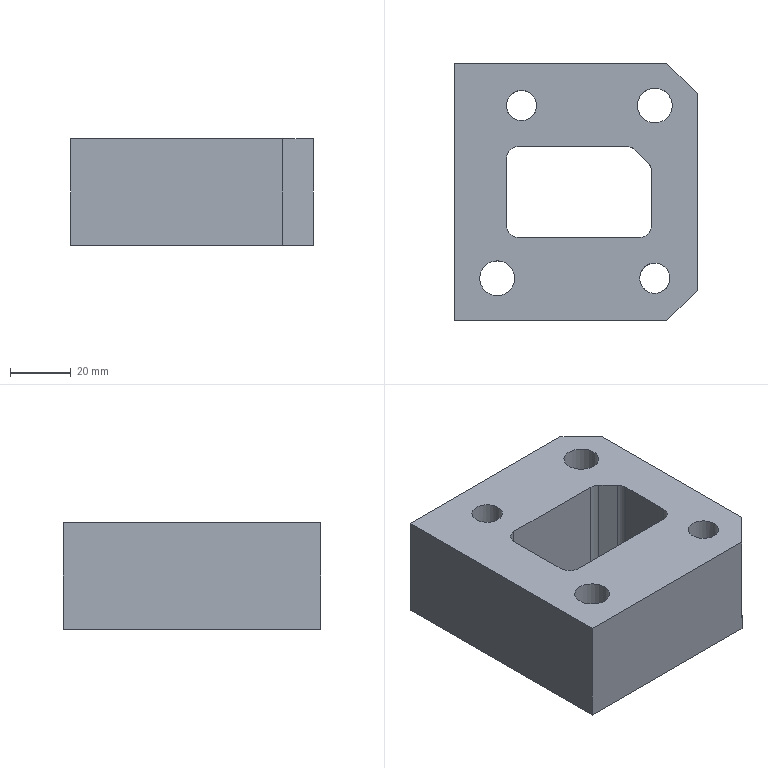Part | NX | features 7 2 | 1 solid | 30 faces | box 80 x 85 x 35 mm | volume 168471 mm3 | plane 17 | cylinder 13 | commonest cylinder face diameters 8 x5 10.001 x2 10.31 x2 11.5 x2 18 x2
STEP:
#1=CARTESIAN_POINT('',(-6.694,33.501,91.));
#2=VERTEX_POINT('',#1);
#3=CARTESIAN_POINT('',(-6.694,28.5,91.));
#4=DIRECTION('',(0.,0.,1.));
#5=DIRECTION('',(0.,1.,0.));
#6=AXIS2_PLACEMENT_3D('',#3,#4,#5);
#7=CIRCLE('',#6,5.);
#8=EDGE_CURVE('',#2,#2,#7,.T.);
#9=ORIENTED_EDGE('',*,*,#8,.F.);
#10=EDGE_LOOP('',(#9));
#11=FACE_BOUND('',#10,.T.);
#12=CARTESIAN_POINT('',(37.306,34.25,91.));
#13=VERTEX_POINT('',#12);
#14=CARTESIAN_POINT('',(37.306,28.5,91.));
#15=DIRECTION('',(0.,0.,-1.));
#16=DIRECTION('',(0.,1.,0.));
#17=AXIS2_PLACEMENT_3D('',#14,#15,#16);
#18=CIRCLE('',#17,5.75);
#19=EDGE_CURVE('',#13,#13,#18,.T.);
#20=ORIENTED_EDGE('',*,*,#19,.T.);
#21=EDGE_LOOP('',(#20));
#22=FACE_BOUND('',#21,.T.);
#23=CARTESIAN_POINT('',(-28.694,-42.5,91.));
#24=VERTEX_POINT('',#23);
#25=CARTESIAN_POINT('',(41.306,-42.5,91.));
#26=VERTEX_POINT('',#25);
#27=CARTESIAN_POINT('',(21.306,-42.5,91.));
#28=DIRECTION('',(1.,0.,0.));
#29=VECTOR('',#28,1000.);
#30=LINE('',#27,#29);
#31=EDGE_CURVE('',#24,#26,#30,.T.);
#32=ORIENTED_EDGE('',*,*,#31,.T.);
#33=CARTESIAN_POINT('',(51.306,-32.5,91.));
#34=VERTEX_POINT('',#33);
#35=CARTESIAN_POINT('',(52.556,-31.25,91.));
#36=DIRECTION('',(0.7071,0.7071,0.));
#37=VECTOR('',#36,1000.);
#38=LINE('',#35,#37);
#39=EDGE_CURVE('',#26,#34,#38,.T.);
#40=ORIENTED_EDGE('',*,*,#39,.T.);
#41=CARTESIAN_POINT('',(51.306,32.5,91.));
#42=VERTEX_POINT('',#41);
#43=CARTESIAN_POINT('',(51.306,0.,91.));
#44=DIRECTION('',(0.,1.,0.));
#45=VECTOR('',#44,1000.);
#46=LINE('',#43,#45);
#47=EDGE_CURVE('',#34,#42,#46,.T.);
#48=ORIENTED_EDGE('',*,*,#47,.T.);
#49=CARTESIAN_POINT('',(41.306,42.5,91.));
#50=VERTEX_POINT('',#49);
#51=CARTESIAN_POINT('',(52.556,31.25,91.));
#52=DIRECTION('',(-0.7071,0.7071,0.));
#53=VECTOR('',#52,1000.);
#54=LINE('',#51,#53);
#55=EDGE_CURVE('',#42,#50,#54,.T.);
#56=ORIENTED_EDGE('',*,*,#55,.T.);
#57=CARTESIAN_POINT('',(-28.694,42.5,91.));
#58=VERTEX_POINT('',#57);
#59=CARTESIAN_POINT('',(21.306,42.5,91.));
#60=DIRECTION('',(-1.,0.,0.));
#61=VECTOR('',#60,1000.);
#62=LINE('',#59,#61);
#63=EDGE_CURVE('',#50,#58,#62,.T.);
#64=ORIENTED_EDGE('',*,*,#63,.T.);
#65=CARTESIAN_POINT('',(-28.694,0.,91.));
#66=DIRECTION('',(0.,-1.,0.));
#67=VECTOR('',#66,1000.);
#68=LINE('',#65,#67);
#69=EDGE_CURVE('',#58,#24,#68,.T.);
#70=ORIENTED_EDGE('',*,*,#69,.T.);
#71=EDGE_LOOP('',(#32,#40,#48,#56,#64,#70));
#72=FACE_BOUND('',#71,.T.);
#73=CARTESIAN_POINT('',(-14.694,-22.75,91.));
#74=VERTEX_POINT('',#73);
#75=CARTESIAN_POINT('',(-14.694,-28.5,91.));
#76=DIRECTION('',(0.,0.,-1.));
#77=DIRECTION('',(0.,1.,0.));
#78=AXIS2_PLACEMENT_3D('',#75,#76,#77);
#79=CIRCLE('',#78,5.75);
#80=EDGE_CURVE('',#74,#74,#79,.T.);
#81=ORIENTED_EDGE('',*,*,#80,.T.);
#82=EDGE_LOOP('',(#81));
#83=FACE_BOUND('',#82,.T.);
#84=CARTESIAN_POINT('',(37.306,-23.499,91.));
#85=VERTEX_POINT('',#84);
#86=CARTESIAN_POINT('',(37.306,-28.5,91.));
#87=DIRECTION('',(0.,0.,1.));
#88=DIRECTION('',(0.,1.,0.));
#89=AXIS2_PLACEMENT_3D('',#86,#87,#88);
#90=CIRCLE('',#89,5.);
#91=EDGE_CURVE('',#85,#85,#90,.T.);
#92=ORIENTED_EDGE('',*,*,#91,.F.);
#93=EDGE_LOOP('',(#92));
#94=FACE_BOUND('',#93,.T.);
#95=CARTESIAN_POINT('',(-7.694,-15.,91.));
#96=VERTEX_POINT('',#95);
#97=CARTESIAN_POINT('',(-11.694,-11.,91.));
#98=VERTEX_POINT('',#97);
#99=CARTESIAN_POINT('',(-7.694,-11.,91.));
#100=DIRECTION('',(0.,0.,-1.));
#101=DIRECTION('',(0.,1.,0.));
#102=AXIS2_PLACEMENT_3D('',#99,#100,#101);
#103=CIRCLE('',#102,4.);
#104=EDGE_CURVE('',#96,#98,#103,.T.);
#105=ORIENTED_EDGE('',*,*,#104,.T.);
#106=CARTESIAN_POINT('',(-11.694,11.,91.));
#107=VERTEX_POINT('',#106);
#108=CARTESIAN_POINT('',(-11.694,0.,91.));
#109=DIRECTION('',(0.,-1.,0.));
#110=VECTOR('',#109,1000.);
#111=LINE('',#108,#110);
#112=EDGE_CURVE('',#107,#98,#111,.T.);
#113=ORIENTED_EDGE('',*,*,#112,.F.);
#114=CARTESIAN_POINT('',(-7.694,15.,91.));
#115=VERTEX_POINT('',#114);
#116=CARTESIAN_POINT('',(-7.694,11.,91.));
#117=DIRECTION('',(0.,0.,-1.));
#118=DIRECTION('',(0.,1.,0.));
#119=AXIS2_PLACEMENT_3D('',#116,#117,#118);
#120=CIRCLE('',#119,4.);
#121=EDGE_CURVE('',#107,#115,#120,.T.);
#122=ORIENTED_EDGE('',*,*,#121,.T.);
#123=CARTESIAN_POINT('',(28.013,15.,91.));
#124=VERTEX_POINT('',#123);
#125=CARTESIAN_POINT('',(21.306,15.,91.));
#126=DIRECTION('',(-1.,0.,0.));
#127=VECTOR('',#126,1000.);
#128=LINE('',#125,#127);
#129=EDGE_CURVE('',#124,#115,#128,.T.);
#130=ORIENTED_EDGE('',*,*,#129,.F.);
#131=CARTESIAN_POINT('',(30.842,13.828,91.));
#132=VERTEX_POINT('',#131);
#133=CARTESIAN_POINT('',(28.013,11.,91.));
#134=DIRECTION('',(0.,0.,-1.));
#135=DIRECTION('',(0.,1.,0.));
#136=AXIS2_PLACEMENT_3D('',#133,#134,#135);
#137=CIRCLE('',#136,4.);
#138=EDGE_CURVE('',#124,#132,#137,.T.);
#139=ORIENTED_EDGE('',*,*,#138,.T.);
#140=CARTESIAN_POINT('',(35.135,9.536,91.));
#141=VERTEX_POINT('',#140);
#142=CARTESIAN_POINT('',(31.738,12.932,91.));
#143=DIRECTION('',(0.7071,-0.7071,0.));
#144=VECTOR('',#143,1000.);
#145=LINE('',#142,#144);
#146=EDGE_CURVE('',#132,#141,#145,.T.);
#147=ORIENTED_EDGE('',*,*,#146,.T.);
#148=CARTESIAN_POINT('',(36.306,6.707,91.));
#149=VERTEX_POINT('',#148);
#150=CARTESIAN_POINT('',(32.306,6.707,91.));
#151=DIRECTION('',(0.,0.,-1.));
#152=DIRECTION('',(0.,1.,0.));
#153=AXIS2_PLACEMENT_3D('',#150,#151,#152);
#154=CIRCLE('',#153,4.);
#155=EDGE_CURVE('',#141,#149,#154,.T.);
#156=ORIENTED_EDGE('',*,*,#155,.T.);
#157=CARTESIAN_POINT('',(36.306,-11.,91.));
#158=VERTEX_POINT('',#157);
#159=CARTESIAN_POINT('',(36.306,0.,91.));
#160=DIRECTION('',(0.,1.,0.));
#161=VECTOR('',#160,1000.);
#162=LINE('',#159,#161);
#163=EDGE_CURVE('',#158,#149,#162,.T.);
#164=ORIENTED_EDGE('',*,*,#163,.F.);
#165=CARTESIAN_POINT('',(32.306,-15.,91.));
#166=VERTEX_POINT('',#165);
#167=CARTESIAN_POINT('',(32.306,-11.,91.));
#168=DIRECTION('',(0.,0.,-1.));
#169=DIRECTION('',(0.,1.,0.));
#170=AXIS2_PLACEMENT_3D('',#167,#168,#169);
#171=CIRCLE('',#170,4.);
#172=EDGE_CURVE('',#158,#166,#171,.T.);
#173=ORIENTED_EDGE('',*,*,#172,.T.);
#174=CARTESIAN_POINT('',(21.306,-15.,91.));
#175=DIRECTION('',(1.,0.,0.));
#176=VECTOR('',#175,1000.);
#177=LINE('',#174,#176);
#178=EDGE_CURVE('',#96,#166,#177,.T.);
#179=ORIENTED_EDGE('',*,*,#178,.F.);
#180=EDGE_LOOP('',(#105,#113,#122,#130,#139,#147,#156,#164,#173,#179));
#181=FACE_BOUND('',#180,.T.);
#182=CARTESIAN_POINT('',(21.306,0.,91.));
#183=DIRECTION('',(0.,0.,1.));
#184=DIRECTION('',(0.,-1.,0.));
#185=AXIS2_PLACEMENT_3D('',#182,#183,#184);
#186=PLANE('',#185);
#187=ADVANCED_FACE('',(#11,#22,#72,#83,#94,#181),#186,.T.);
#188=CARTESIAN_POINT('',(42.461,-28.5,56.));
#189=VERTEX_POINT('',#188);
#190=CARTESIAN_POINT('',(37.306,-28.5,56.));
#191=DIRECTION('',(0.,0.,1.));
#192=DIRECTION('',(1.,0.,0.));
#193=AXIS2_PLACEMENT_3D('',#190,#191,#192);
#194=CIRCLE('',#193,5.155);
#195=EDGE_CURVE('',#189,#189,#194,.T.);
#196=ORIENTED_EDGE('',*,*,#195,.T.);
#197=EDGE_LOOP('',(#196));
#198=FACE_BOUND('',#197,.T.);
#199=CARTESIAN_POINT('',(-1.539,28.5,56.));
#200=VERTEX_POINT('',#199);
#201=CARTESIAN_POINT('',(-6.694,28.5,56.));
#202=DIRECTION('',(0.,0.,1.));
#203=DIRECTION('',(1.,0.,0.));
#204=AXIS2_PLACEMENT_3D('',#201,#202,#203);
#205=CIRCLE('',#204,5.155);
#206=EDGE_CURVE('',#200,#200,#205,.T.);
#207=ORIENTED_EDGE('',*,*,#206,.T.);
#208=EDGE_LOOP('',(#207));
#209=FACE_BOUND('',#208,.T.);
#210=CARTESIAN_POINT('',(51.306,32.5,56.));
#211=VERTEX_POINT('',#210);
#212=CARTESIAN_POINT('',(51.306,-32.5,56.));
#213=VERTEX_POINT('',#212);
#214=CARTESIAN_POINT('',(51.306,0.,56.));
#215=DIRECTION('',(0.,-1.,0.));
#216=VECTOR('',#215,1000.);
#217=LINE('',#214,#216);
#218=EDGE_CURVE('',#211,#213,#217,.T.);
#219=ORIENTED_EDGE('',*,*,#218,.T.);
#220=CARTESIAN_POINT('',(41.306,-42.5,56.));
#221=VERTEX_POINT('',#220);
#222=CARTESIAN_POINT('',(-128.444,-212.25,56.));
#223=DIRECTION('',(-0.7071,-0.7071,0.));
#224=VECTOR('',#223,1000.);
#225=LINE('',#222,#224);
#226=EDGE_CURVE('',#213,#221,#225,.T.);
#227=ORIENTED_EDGE('',*,*,#226,.T.);
#228=CARTESIAN_POINT('',(-28.694,-42.5,56.));
#229=VERTEX_POINT('',#228);
#230=CARTESIAN_POINT('',(21.306,-42.5,56.));
#231=DIRECTION('',(-1.,0.,0.));
#232=VECTOR('',#231,1000.);
#233=LINE('',#230,#232);
#234=EDGE_CURVE('',#221,#229,#233,.T.);
#235=ORIENTED_EDGE('',*,*,#234,.T.);
#236=CARTESIAN_POINT('',(-28.694,42.5,56.));
#237=VERTEX_POINT('',#236);
#238=CARTESIAN_POINT('',(-28.694,0.,56.));
#239=DIRECTION('',(0.,1.,0.));
#240=VECTOR('',#239,1000.);
#241=LINE('',#238,#240);
#242=EDGE_CURVE('',#229,#237,#241,.T.);
#243=ORIENTED_EDGE('',*,*,#242,.T.);
#244=CARTESIAN_POINT('',(41.306,42.5,56.));
#245=VERTEX_POINT('',#244);
#246=CARTESIAN_POINT('',(21.306,42.5,56.));
#247=DIRECTION('',(1.,0.,0.));
#248=VECTOR('',#247,1000.);
#249=LINE('',#246,#248);
#250=EDGE_CURVE('',#237,#245,#249,.T.);
#251=ORIENTED_EDGE('',*,*,#250,.T.);
#252=CARTESIAN_POINT('',(48.556,35.25,56.));
#253=DIRECTION('',(0.7071,-0.7071,0.));
#254=VECTOR('',#253,1000.);
#255=LINE('',#252,#254);
#256=EDGE_CURVE('',#245,#211,#255,.T.);
#257=ORIENTED_EDGE('',*,*,#256,.T.);
#258=EDGE_LOOP('',(#219,#227,#235,#243,#251,#257));
#259=FACE_BOUND('',#258,.T.);
#260=CARTESIAN_POINT('',(-14.694,-37.5,56.));
#261=VERTEX_POINT('',#260);
#262=CARTESIAN_POINT('',(-14.694,-28.5,56.));
#263=DIRECTION('',(0.,0.,-1.));
#264=DIRECTION('',(0.,-1.,0.));
#265=AXIS2_PLACEMENT_3D('',#262,#263,#264);
#266=CIRCLE('',#265,9.);
#267=EDGE_CURVE('',#261,#261,#266,.T.);
#268=ORIENTED_EDGE('',*,*,#267,.F.);
#269=EDGE_LOOP('',(#268));
#270=FACE_BOUND('',#269,.T.);
#271=CARTESIAN_POINT('',(37.306,19.5,56.));
#272=VERTEX_POINT('',#271);
#273=CARTESIAN_POINT('',(37.306,28.5,56.));
#274=DIRECTION('',(0.,0.,-1.));
#275=DIRECTION('',(0.,-1.,0.));
#276=AXIS2_PLACEMENT_3D('',#273,#274,#275);
#277=CIRCLE('',#276,9.);
#278=EDGE_CURVE('',#272,#272,#277,.T.);
#279=ORIENTED_EDGE('',*,*,#278,.F.);
#280=EDGE_LOOP('',(#279));
#281=FACE_BOUND('',#280,.T.);
#282=CARTESIAN_POINT('',(-11.694,-11.,56.));
#283=VERTEX_POINT('',#282);
#284=CARTESIAN_POINT('',(-7.694,-15.,56.));
#285=VERTEX_POINT('',#284);
#286=CARTESIAN_POINT('',(-7.694,-11.,56.));
#287=DIRECTION('',(0.,0.,1.));
#288=DIRECTION('',(0.,-1.,0.));
#289=AXIS2_PLACEMENT_3D('',#286,#287,#288);
#290=CIRCLE('',#289,4.);
#291=EDGE_CURVE('',#283,#285,#290,.T.);
#292=ORIENTED_EDGE('',*,*,#291,.T.);
#293=CARTESIAN_POINT('',(32.306,-15.,56.));
#294=VERTEX_POINT('',#293);
#295=CARTESIAN_POINT('',(21.306,-15.,56.));
#296=DIRECTION('',(-1.,0.,0.));
#297=VECTOR('',#296,1000.);
#298=LINE('',#295,#297);
#299=EDGE_CURVE('',#294,#285,#298,.T.);
#300=ORIENTED_EDGE('',*,*,#299,.F.);
#301=CARTESIAN_POINT('',(36.306,-11.,56.));
#302=VERTEX_POINT('',#301);
#303=CARTESIAN_POINT('',(32.306,-11.,56.));
#304=DIRECTION('',(0.,0.,1.));
#305=DIRECTION('',(0.,-1.,0.));
#306=AXIS2_PLACEMENT_3D('',#303,#304,#305);
#307=CIRCLE('',#306,4.);
#308=EDGE_CURVE('',#294,#302,#307,.T.);
#309=ORIENTED_EDGE('',*,*,#308,.T.);
#310=CARTESIAN_POINT('',(36.306,6.707,56.));
#311=VERTEX_POINT('',#310);
#312=CARTESIAN_POINT('',(36.306,0.,56.));
#313=DIRECTION('',(0.,-1.,0.));
#314=VECTOR('',#313,1000.);
#315=LINE('',#312,#314);
#316=EDGE_CURVE('',#311,#302,#315,.T.);
#317=ORIENTED_EDGE('',*,*,#316,.F.);
#318=CARTESIAN_POINT('',(35.135,9.536,56.));
#319=VERTEX_POINT('',#318);
#320=CARTESIAN_POINT('',(32.306,6.707,56.));
#321=DIRECTION('',(0.,0.,1.));
#322=DIRECTION('',(0.,-1.,0.));
#323=AXIS2_PLACEMENT_3D('',#320,#321,#322);
#324=CIRCLE('',#323,4.);
#325=EDGE_CURVE('',#311,#319,#324,.T.);
#326=ORIENTED_EDGE('',*,*,#325,.T.);
#327=CARTESIAN_POINT('',(30.842,13.828,56.));
#328=VERTEX_POINT('',#327);
#329=CARTESIAN_POINT('',(28.988,15.682,56.));
#330=DIRECTION('',(-0.7071,0.7071,0.));
#331=VECTOR('',#330,1000.);
#332=LINE('',#329,#331);
#333=EDGE_CURVE('',#319,#328,#332,.T.);
#334=ORIENTED_EDGE('',*,*,#333,.T.);
#335=CARTESIAN_POINT('',(28.013,15.,56.));
#336=VERTEX_POINT('',#335);
#337=CARTESIAN_POINT('',(28.013,11.,56.));
#338=DIRECTION('',(0.,0.,1.));
#339=DIRECTION('',(0.,-1.,0.));
#340=AXIS2_PLACEMENT_3D('',#337,#338,#339);
#341=CIRCLE('',#340,4.);
#342=EDGE_CURVE('',#328,#336,#341,.T.);
#343=ORIENTED_EDGE('',*,*,#342,.T.);
#344=CARTESIAN_POINT('',(-7.694,15.,56.));
#345=VERTEX_POINT('',#344);
#346=CARTESIAN_POINT('',(21.306,15.,56.));
#347=DIRECTION('',(1.,0.,0.));
#348=VECTOR('',#347,1000.);
#349=LINE('',#346,#348);
#350=EDGE_CURVE('',#345,#336,#349,.T.);
#351=ORIENTED_EDGE('',*,*,#350,.F.);
#352=CARTESIAN_POINT('',(-11.694,11.,56.));
#353=VERTEX_POINT('',#352);
#354=CARTESIAN_POINT('',(-7.694,11.,56.));
#355=DIRECTION('',(0.,0.,1.));
#356=DIRECTION('',(0.,-1.,0.));
#357=AXIS2_PLACEMENT_3D('',#354,#355,#356);
#358=CIRCLE('',#357,4.);
#359=EDGE_CURVE('',#345,#353,#358,.T.);
#360=ORIENTED_EDGE('',*,*,#359,.T.);
#361=CARTESIAN_POINT('',(-11.694,0.,56.));
#362=DIRECTION('',(0.,1.,0.));
#363=VECTOR('',#362,1000.);
#364=LINE('',#361,#363);
#365=EDGE_CURVE('',#283,#353,#364,.T.);
#366=ORIENTED_EDGE('',*,*,#365,.F.);
#367=EDGE_LOOP('',(#292,#300,#309,#317,#326,#334,#343,#351,#360,#366));
#368=FACE_BOUND('',#367,.T.);
#369=CARTESIAN_POINT('',(-163.694,-177.,56.));
#370=DIRECTION('',(0.,0.,-1.));
#371=DIRECTION('',(0.,1.,0.));
#372=AXIS2_PLACEMENT_3D('',#369,#370,#371);
#373=PLANE('',#372);
#374=ADVANCED_FACE('',(#198,#209,#259,#270,#281,#368),#373,.T.);
#375=ORIENTED_EDGE('',*,*,#47,.F.);
#376=CARTESIAN_POINT('',(51.306,-32.5,6.933));
#377=DIRECTION('',(0.,0.,-1.));
#378=VECTOR('',#377,1000.);
#379=LINE('',#376,#378);
#380=EDGE_CURVE('',#34,#213,#379,.T.);
#381=ORIENTED_EDGE('',*,*,#380,.T.);
#382=ORIENTED_EDGE('',*,*,#218,.F.);
#383=CARTESIAN_POINT('',(51.306,32.5,6.933));
#384=DIRECTION('',(0.,0.,1.));
#385=VECTOR('',#384,1000.);
#386=LINE('',#383,#385);
#387=EDGE_CURVE('',#211,#42,#386,.T.);
#388=ORIENTED_EDGE('',*,*,#387,.T.);
#389=EDGE_LOOP('',(#375,#381,#382,#388));
#390=FACE_BOUND('',#389,.T.);
#391=CARTESIAN_POINT('',(51.306,0.,6.933));
#392=DIRECTION('',(1.,0.,0.));
#393=DIRECTION('',(0.,0.,-1.));
#394=AXIS2_PLACEMENT_3D('',#391,#392,#393);
#395=PLANE('',#394);
#396=ADVANCED_FACE('',(#390),#395,.T.);
#397=ORIENTED_EDGE('',*,*,#63,.F.);
#398=CARTESIAN_POINT('',(41.306,42.5,6.933));
#399=DIRECTION('',(0.,0.,-1.));
#400=VECTOR('',#399,1000.);
#401=LINE('',#398,#400);
#402=EDGE_CURVE('',#50,#245,#401,.T.);
#403=ORIENTED_EDGE('',*,*,#402,.T.);
#404=ORIENTED_EDGE('',*,*,#250,.F.);
#405=CARTESIAN_POINT('',(-28.694,42.5,6.933));
#406=DIRECTION('',(0.,0.,-1.));
#407=VECTOR('',#406,1000.);
#408=LINE('',#405,#407);
#409=EDGE_CURVE('',#58,#237,#408,.T.);
#410=ORIENTED_EDGE('',*,*,#409,.F.);
#411=EDGE_LOOP('',(#397,#403,#404,#410));
#412=FACE_BOUND('',#411,.T.);
#413=CARTESIAN_POINT('',(21.306,42.5,6.933));
#414=DIRECTION('',(0.,1.,0.));
#415=DIRECTION('',(0.,0.,1.));
#416=AXIS2_PLACEMENT_3D('',#413,#414,#415);
#417=PLANE('',#416);
#418=ADVANCED_FACE('',(#412),#417,.T.);
#419=ORIENTED_EDGE('',*,*,#69,.F.);
#420=ORIENTED_EDGE('',*,*,#409,.T.);
#421=ORIENTED_EDGE('',*,*,#242,.F.);
#422=CARTESIAN_POINT('',(-28.694,-42.5,6.933));
#423=DIRECTION('',(0.,0.,1.));
#424=VECTOR('',#423,1000.);
#425=LINE('',#422,#424);
#426=EDGE_CURVE('',#229,#24,#425,.T.);
#427=ORIENTED_EDGE('',*,*,#426,.T.);
#428=EDGE_LOOP('',(#419,#420,#421,#427));
#429=FACE_BOUND('',#428,.T.);
#430=CARTESIAN_POINT('',(-28.694,0.,6.933));
#431=DIRECTION('',(-1.,0.,0.));
#432=DIRECTION('',(0.,0.,1.));
#433=AXIS2_PLACEMENT_3D('',#430,#431,#432);
#434=PLANE('',#433);
#435=ADVANCED_FACE('',(#429),#434,.T.);
#436=ORIENTED_EDGE('',*,*,#234,.F.);
#437=CARTESIAN_POINT('',(41.306,-42.5,6.933));
#438=DIRECTION('',(0.,0.,1.));
#439=VECTOR('',#438,1000.);
#440=LINE('',#437,#439);
#441=EDGE_CURVE('',#221,#26,#440,.T.);
#442=ORIENTED_EDGE('',*,*,#441,.T.);
#443=ORIENTED_EDGE('',*,*,#31,.F.);
#444=ORIENTED_EDGE('',*,*,#426,.F.);
#445=EDGE_LOOP('',(#436,#442,#443,#444));
#446=FACE_BOUND('',#445,.T.);
#447=CARTESIAN_POINT('',(21.306,-42.5,6.933));
#448=DIRECTION('',(0.,-1.,0.));
#449=DIRECTION('',(0.,0.,-1.));
#450=AXIS2_PLACEMENT_3D('',#447,#448,#449);
#451=PLANE('',#450);
#452=ADVANCED_FACE('',(#446),#451,.T.);
#453=ORIENTED_EDGE('',*,*,#80,.F.);
#454=EDGE_LOOP('',(#453));
#455=FACE_BOUND('',#454,.T.);
#456=CARTESIAN_POINT('',(-14.694,-22.75,69.));
#457=VERTEX_POINT('',#456);
#458=CARTESIAN_POINT('',(-14.694,-28.5,69.));
#459=DIRECTION('',(0.,0.,-1.));
#460=DIRECTION('',(0.,1.,0.));
#461=AXIS2_PLACEMENT_3D('',#458,#459,#460);
#462=CIRCLE('',#461,5.75);
#463=EDGE_CURVE('',#457,#457,#462,.T.);
#464=ORIENTED_EDGE('',*,*,#463,.T.);
#465=EDGE_LOOP('',(#464));
#466=FACE_BOUND('',#465,.T.);
#467=CARTESIAN_POINT('',(-14.694,-28.5,51.));
#468=DIRECTION('',(0.,0.,1.));
#469=DIRECTION('',(0.,-1.,0.));
#470=AXIS2_PLACEMENT_3D('',#467,#468,#469);
#471=CYLINDRICAL_SURFACE('',#470,5.75);
#472=ADVANCED_FACE('',(#455,#466),#471,.F.);
#473=ORIENTED_EDGE('',*,*,#463,.F.);
#474=EDGE_LOOP('',(#473));
#475=FACE_BOUND('',#474,.T.);
#476=CARTESIAN_POINT('',(-14.694,-19.5,69.));
#477=VERTEX_POINT('',#476);
#478=CARTESIAN_POINT('',(-14.694,-28.5,69.));
#479=DIRECTION('',(0.,0.,-1.));
#480=DIRECTION('',(0.,1.,0.));
#481=AXIS2_PLACEMENT_3D('',#478,#479,#480);
#482=CIRCLE('',#481,9.);
#483=EDGE_CURVE('',#477,#477,#482,.T.);
#484=ORIENTED_EDGE('',*,*,#483,.T.);
#485=EDGE_LOOP('',(#484));
#486=FACE_BOUND('',#485,.T.);
#487=CARTESIAN_POINT('',(-14.694,-28.5,69.));
#488=DIRECTION('',(0.,0.,1.));
#489=DIRECTION('',(0.,-1.,0.));
#490=AXIS2_PLACEMENT_3D('',#487,#488,#489);
#491=PLANE('',#490);
#492=ADVANCED_FACE('',(#475,#486),#491,.F.);
#493=ORIENTED_EDGE('',*,*,#483,.F.);
#494=EDGE_LOOP('',(#493));
#495=FACE_BOUND('',#494,.T.);
#496=ORIENTED_EDGE('',*,*,#267,.T.);
#497=EDGE_LOOP('',(#496));
#498=FACE_BOUND('',#497,.T.);
#499=CARTESIAN_POINT('',(-14.694,-28.5,56.));
#500=DIRECTION('',(0.,0.,1.));
#501=DIRECTION('',(0.,-1.,0.));
#502=AXIS2_PLACEMENT_3D('',#499,#500,#501);
#503=CYLINDRICAL_SURFACE('',#502,9.);
#504=ADVANCED_FACE('',(#495,#498),#503,.F.);
#505=CARTESIAN_POINT('',(42.307,-28.5,66.));
#506=VERTEX_POINT('',#505);
#507=CARTESIAN_POINT('',(37.306,-28.5,66.));
#508=DIRECTION('',(0.,0.,-1.));
#509=DIRECTION('',(1.,0.,0.));
#510=AXIS2_PLACEMENT_3D('',#507,#508,#509);
#511=CIRCLE('',#510,5.);
#512=EDGE_CURVE('',#506,#506,#511,.T.);
#513=ORIENTED_EDGE('',*,*,#512,.T.);
#514=EDGE_LOOP('',(#513));
#515=FACE_BOUND('',#514,.T.);
#516=ORIENTED_EDGE('',*,*,#91,.T.);
#517=EDGE_LOOP('',(#516));
#518=FACE_BOUND('',#517,.T.);
#519=CARTESIAN_POINT('',(37.306,-28.5,621.));
#520=DIRECTION('',(0.,0.,-1.));
#521=DIRECTION('',(0.,1.,0.));
#522=AXIS2_PLACEMENT_3D('',#519,#520,#521);
#523=CYLINDRICAL_SURFACE('',#522,5.);
#524=ADVANCED_FACE('',(#515,#518),#523,.F.);
#525=ORIENTED_EDGE('',*,*,#19,.F.);
#526=EDGE_LOOP('',(#525));
#527=FACE_BOUND('',#526,.T.);
#528=CARTESIAN_POINT('',(37.306,34.25,69.));
#529=VERTEX_POINT('',#528);
#530=CARTESIAN_POINT('',(37.306,28.5,69.));
#531=DIRECTION('',(0.,0.,-1.));
#532=DIRECTION('',(0.,1.,0.));
#533=AXIS2_PLACEMENT_3D('',#530,#531,#532);
#534=CIRCLE('',#533,5.75);
#535=EDGE_CURVE('',#529,#529,#534,.T.);
#536=ORIENTED_EDGE('',*,*,#535,.T.);
#537=EDGE_LOOP('',(#536));
#538=FACE_BOUND('',#537,.T.);
#539=CARTESIAN_POINT('',(37.306,28.5,51.));
#540=DIRECTION('',(0.,0.,1.));
#541=DIRECTION('',(0.,-1.,0.));
#542=AXIS2_PLACEMENT_3D('',#539,#540,#541);
#543=CYLINDRICAL_SURFACE('',#542,5.75);
#544=ADVANCED_FACE('',(#527,#538),#543,.F.);
#545=ORIENTED_EDGE('',*,*,#535,.F.);
#546=EDGE_LOOP('',(#545));
#547=FACE_BOUND('',#546,.T.);
#548=CARTESIAN_POINT('',(37.306,37.5,69.));
#549=VERTEX_POINT('',#548);
#550=CARTESIAN_POINT('',(37.306,28.5,69.));
#551=DIRECTION('',(0.,0.,-1.));
#552=DIRECTION('',(0.,1.,0.));
#553=AXIS2_PLACEMENT_3D('',#550,#551,#552);
#554=CIRCLE('',#553,9.);
#555=EDGE_CURVE('',#549,#549,#554,.T.);
#556=ORIENTED_EDGE('',*,*,#555,.T.);
#557=EDGE_LOOP('',(#556));
#558=FACE_BOUND('',#557,.T.);
#559=CARTESIAN_POINT('',(37.306,28.5,69.));
#560=DIRECTION('',(0.,0.,1.));
#561=DIRECTION('',(0.,-1.,0.));
#562=AXIS2_PLACEMENT_3D('',#559,#560,#561);
#563=PLANE('',#562);
#564=ADVANCED_FACE('',(#547,#558),#563,.F.);
#565=ORIENTED_EDGE('',*,*,#555,.F.);
#566=EDGE_LOOP('',(#565));
#567=FACE_BOUND('',#566,.T.);
#568=ORIENTED_EDGE('',*,*,#278,.T.);
#569=EDGE_LOOP('',(#568));
#570=FACE_BOUND('',#569,.T.);
#571=CARTESIAN_POINT('',(37.306,28.5,56.));
#572=DIRECTION('',(0.,0.,1.));
#573=DIRECTION('',(0.,-1.,0.));
#574=AXIS2_PLACEMENT_3D('',#571,#572,#573);
#575=CYLINDRICAL_SURFACE('',#574,9.);
#576=ADVANCED_FACE('',(#567,#570),#575,.F.);
#577=CARTESIAN_POINT('',(-1.693,28.5,66.));
#578=VERTEX_POINT('',#577);
#579=CARTESIAN_POINT('',(-6.694,28.5,66.));
#580=DIRECTION('',(0.,0.,-1.));
#581=DIRECTION('',(1.,0.,0.));
#582=AXIS2_PLACEMENT_3D('',#579,#580,#581);
#583=CIRCLE('',#582,5.);
#584=EDGE_CURVE('',#578,#578,#583,.T.);
#585=ORIENTED_EDGE('',*,*,#584,.T.);
#586=EDGE_LOOP('',(#585));
#587=FACE_BOUND('',#586,.T.);
#588=ORIENTED_EDGE('',*,*,#8,.T.);
#589=EDGE_LOOP('',(#588));
#590=FACE_BOUND('',#589,.T.);
#591=CARTESIAN_POINT('',(-6.694,28.5,621.));
#592=DIRECTION('',(0.,0.,-1.));
#593=DIRECTION('',(0.,1.,0.));
#594=AXIS2_PLACEMENT_3D('',#591,#592,#593);
#595=CYLINDRICAL_SURFACE('',#594,5.);
#596=ADVANCED_FACE('',(#587,#590),#595,.F.);
#597=ORIENTED_EDGE('',*,*,#163,.T.);
#598=CARTESIAN_POINT('',(36.306,6.707,-5.));
#599=DIRECTION('',(0.,0.,1.));
#600=VECTOR('',#599,1000.);
#601=LINE('',#598,#600);
#602=EDGE_CURVE('',#311,#149,#601,.T.);
#603=ORIENTED_EDGE('',*,*,#602,.F.);
#604=ORIENTED_EDGE('',*,*,#316,.T.);
#605=CARTESIAN_POINT('',(36.306,-11.,-5.));
#606=DIRECTION('',(0.,0.,-1.));
#607=VECTOR('',#606,1000.);
#608=LINE('',#605,#607);
#609=EDGE_CURVE('',#158,#302,#608,.T.);
#610=ORIENTED_EDGE('',*,*,#609,.F.);
#611=EDGE_LOOP('',(#597,#603,#604,#610));
#612=FACE_BOUND('',#611,.T.);
#613=CARTESIAN_POINT('',(36.306,0.,-5.));
#614=DIRECTION('',(1.,0.,0.));
#615=DIRECTION('',(0.,0.,-1.));
#616=AXIS2_PLACEMENT_3D('',#613,#614,#615);
#617=PLANE('',#616);
#618=ADVANCED_FACE('',(#612),#617,.F.);
#619=ORIENTED_EDGE('',*,*,#129,.T.);
#620=CARTESIAN_POINT('',(-7.694,15.,-5.));
#621=DIRECTION('',(0.,0.,1.));
#622=VECTOR('',#621,1000.);
#623=LINE('',#620,#622);
#624=EDGE_CURVE('',#345,#115,#623,.T.);
#625=ORIENTED_EDGE('',*,*,#624,.F.);
#626=ORIENTED_EDGE('',*,*,#350,.T.);
#627=CARTESIAN_POINT('',(28.013,15.,-5.));
#628=DIRECTION('',(0.,0.,-1.));
#629=VECTOR('',#628,1000.);
#630=LINE('',#627,#629);
#631=EDGE_CURVE('',#124,#336,#630,.T.);
#632=ORIENTED_EDGE('',*,*,#631,.F.);
#633=EDGE_LOOP('',(#619,#625,#626,#632));
#634=FACE_BOUND('',#633,.T.);
#635=CARTESIAN_POINT('',(21.306,15.,-5.));
#636=DIRECTION('',(0.,1.,0.));
#637=DIRECTION('',(0.,0.,1.));
#638=AXIS2_PLACEMENT_3D('',#635,#636,#637);
#639=PLANE('',#638);
#640=ADVANCED_FACE('',(#634),#639,.F.);
#641=ORIENTED_EDGE('',*,*,#112,.T.);
#642=CARTESIAN_POINT('',(-11.694,-11.,-5.));
#643=DIRECTION('',(0.,0.,1.));
#644=VECTOR('',#643,1000.);
#645=LINE('',#642,#644);
#646=EDGE_CURVE('',#283,#98,#645,.T.);
#647=ORIENTED_EDGE('',*,*,#646,.F.);
#648=ORIENTED_EDGE('',*,*,#365,.T.);
#649=CARTESIAN_POINT('',(-11.694,11.,-5.));
#650=DIRECTION('',(0.,0.,-1.));
#651=VECTOR('',#650,1000.);
#652=LINE('',#649,#651);
#653=EDGE_CURVE('',#107,#353,#652,.T.);
#654=ORIENTED_EDGE('',*,*,#653,.F.);
#655=EDGE_LOOP('',(#641,#647,#648,#654));
#656=FACE_BOUND('',#655,.T.);
#657=CARTESIAN_POINT('',(-11.694,0.,-5.));
#658=DIRECTION('',(-1.,0.,0.));
#659=DIRECTION('',(0.,0.,1.));
#660=AXIS2_PLACEMENT_3D('',#657,#658,#659);
#661=PLANE('',#660);
#662=ADVANCED_FACE('',(#656),#661,.F.);
#663=ORIENTED_EDGE('',*,*,#299,.T.);
#664=CARTESIAN_POINT('',(-7.694,-15.,-5.));
#665=DIRECTION('',(0.,0.,-1.));
#666=VECTOR('',#665,1000.);
#667=LINE('',#664,#666);
#668=EDGE_CURVE('',#96,#285,#667,.T.);
#669=ORIENTED_EDGE('',*,*,#668,.F.);
#670=ORIENTED_EDGE('',*,*,#178,.T.);
#671=CARTESIAN_POINT('',(32.306,-15.,-5.));
#672=DIRECTION('',(0.,0.,1.));
#673=VECTOR('',#672,1000.);
#674=LINE('',#671,#673);
#675=EDGE_CURVE('',#294,#166,#674,.T.);
#676=ORIENTED_EDGE('',*,*,#675,.F.);
#677=EDGE_LOOP('',(#663,#669,#670,#676));
#678=FACE_BOUND('',#677,.T.);
#679=CARTESIAN_POINT('',(21.306,-15.,-5.));
#680=DIRECTION('',(0.,-1.,0.));
#681=DIRECTION('',(0.,0.,-1.));
#682=AXIS2_PLACEMENT_3D('',#679,#680,#681);
#683=PLANE('',#682);
#684=ADVANCED_FACE('',(#678),#683,.F.);
#685=ORIENTED_EDGE('',*,*,#146,.F.);
#686=CARTESIAN_POINT('',(30.842,13.828,-5.));
#687=DIRECTION('',(0.,0.,1.));
#688=VECTOR('',#687,1000.);
#689=LINE('',#686,#688);
#690=EDGE_CURVE('',#328,#132,#689,.T.);
#691=ORIENTED_EDGE('',*,*,#690,.F.);
#692=ORIENTED_EDGE('',*,*,#333,.F.);
#693=CARTESIAN_POINT('',(35.135,9.536,-5.));
#694=DIRECTION('',(0.,0.,-1.));
#695=VECTOR('',#694,1000.);
#696=LINE('',#693,#695);
#697=EDGE_CURVE('',#141,#319,#696,.T.);
#698=ORIENTED_EDGE('',*,*,#697,.F.);
#699=EDGE_LOOP('',(#685,#691,#692,#698));
#700=FACE_BOUND('',#699,.T.);
#701=CARTESIAN_POINT('',(28.988,15.682,-5.));
#702=DIRECTION('',(-0.7071,-0.7071,0.));
#703=DIRECTION('',(0.,0.,1.));
#704=AXIS2_PLACEMENT_3D('',#701,#702,#703);
#705=PLANE('',#704);
#706=ADVANCED_FACE('',(#700),#705,.T.);
#707=ORIENTED_EDGE('',*,*,#291,.F.);
#708=ORIENTED_EDGE('',*,*,#646,.T.);
#709=ORIENTED_EDGE('',*,*,#104,.F.);
#710=ORIENTED_EDGE('',*,*,#668,.T.);
#711=EDGE_LOOP('',(#707,#708,#709,#710));
#712=FACE_BOUND('',#711,.T.);
#713=CARTESIAN_POINT('',(-7.694,-11.,-5.));
#714=DIRECTION('',(0.,0.,-1.));
#715=DIRECTION('',(0.,-1.,0.));
#716=AXIS2_PLACEMENT_3D('',#713,#714,#715);
#717=CYLINDRICAL_SURFACE('',#716,4.);
#718=ADVANCED_FACE('',(#712),#717,.F.);
#719=ORIENTED_EDGE('',*,*,#359,.F.);
#720=ORIENTED_EDGE('',*,*,#624,.T.);
#721=ORIENTED_EDGE('',*,*,#121,.F.);
#722=ORIENTED_EDGE('',*,*,#653,.T.);
#723=EDGE_LOOP('',(#719,#720,#721,#722));
#724=FACE_BOUND('',#723,.T.);
#725=CARTESIAN_POINT('',(-7.694,11.,-5.));
#726=DIRECTION('',(0.,0.,-1.));
#727=DIRECTION('',(0.,-1.,0.));
#728=AXIS2_PLACEMENT_3D('',#725,#726,#727);
#729=CYLINDRICAL_SURFACE('',#728,4.);
#730=ADVANCED_FACE('',(#724),#729,.F.);
#731=ORIENTED_EDGE('',*,*,#342,.F.);
#732=ORIENTED_EDGE('',*,*,#690,.T.);
#733=ORIENTED_EDGE('',*,*,#138,.F.);
#734=ORIENTED_EDGE('',*,*,#631,.T.);
#735=EDGE_LOOP('',(#731,#732,#733,#734));
#736=FACE_BOUND('',#735,.T.);
#737=CARTESIAN_POINT('',(28.013,11.,-5.));
#738=DIRECTION('',(0.,0.,1.));
#739=DIRECTION('',(0.,1.,0.));
#740=AXIS2_PLACEMENT_3D('',#737,#738,#739);
#741=CYLINDRICAL_SURFACE('',#740,4.);
#742=ADVANCED_FACE('',(#736),#741,.F.);
#743=ORIENTED_EDGE('',*,*,#155,.F.);
#744=ORIENTED_EDGE('',*,*,#697,.T.);
#745=ORIENTED_EDGE('',*,*,#325,.F.);
#746=ORIENTED_EDGE('',*,*,#602,.T.);
#747=EDGE_LOOP('',(#743,#744,#745,#746));
#748=FACE_BOUND('',#747,.T.);
#749=CARTESIAN_POINT('',(32.306,6.707,-5.));
#750=DIRECTION('',(0.,0.,-1.));
#751=DIRECTION('',(0.,-1.,0.));
#752=AXIS2_PLACEMENT_3D('',#749,#750,#751);
#753=CYLINDRICAL_SURFACE('',#752,4.);
#754=ADVANCED_FACE('',(#748),#753,.F.);
#755=ORIENTED_EDGE('',*,*,#308,.F.);
#756=ORIENTED_EDGE('',*,*,#675,.T.);
#757=ORIENTED_EDGE('',*,*,#172,.F.);
#758=ORIENTED_EDGE('',*,*,#609,.T.);
#759=EDGE_LOOP('',(#755,#756,#757,#758));
#760=FACE_BOUND('',#759,.T.);
#761=CARTESIAN_POINT('',(32.306,-11.,-5.));
#762=DIRECTION('',(0.,0.,-1.));
#763=DIRECTION('',(0.,-1.,0.));
#764=AXIS2_PLACEMENT_3D('',#761,#762,#763);
#765=CYLINDRICAL_SURFACE('',#764,4.);
#766=ADVANCED_FACE('',(#760),#765,.F.);
#767=ORIENTED_EDGE('',*,*,#256,.F.);
#768=ORIENTED_EDGE('',*,*,#402,.F.);
#769=ORIENTED_EDGE('',*,*,#55,.F.);
#770=ORIENTED_EDGE('',*,*,#387,.F.);
#771=EDGE_LOOP('',(#767,#768,#769,#770));
#772=FACE_BOUND('',#771,.T.);
#773=CARTESIAN_POINT('',(51.306,32.5,6.933));
#774=DIRECTION('',(-0.7071,-0.7071,0.));
#775=DIRECTION('',(0.,0.,-1.));
#776=AXIS2_PLACEMENT_3D('',#773,#774,#775);
#777=PLANE('',#776);
#778=ADVANCED_FACE('',(#772),#777,.F.);
#779=ORIENTED_EDGE('',*,*,#226,.F.);
#780=ORIENTED_EDGE('',*,*,#380,.F.);
#781=ORIENTED_EDGE('',*,*,#39,.F.);
#782=ORIENTED_EDGE('',*,*,#441,.F.);
#783=EDGE_LOOP('',(#779,#780,#781,#782));
#784=FACE_BOUND('',#783,.T.);
#785=CARTESIAN_POINT('',(41.306,-42.5,6.933));
#786=DIRECTION('',(-0.7071,0.7071,0.));
#787=DIRECTION('',(0.,0.,-1.));
#788=AXIS2_PLACEMENT_3D('',#785,#786,#787);
#789=PLANE('',#788);
#790=ADVANCED_FACE('',(#784),#789,.F.);
#791=CARTESIAN_POINT('',(-1.539,28.5,66.));
#792=VERTEX_POINT('',#791);
#793=CARTESIAN_POINT('',(-6.694,28.5,66.));
#794=DIRECTION('',(0.,0.,-1.));
#795=DIRECTION('',(1.,0.,0.));
#796=AXIS2_PLACEMENT_3D('',#793,#794,#795);
#797=CIRCLE('',#796,5.155);
#798=EDGE_CURVE('',#792,#792,#797,.T.);
#799=ORIENTED_EDGE('',*,*,#798,.T.);
#800=EDGE_LOOP('',(#799));
#801=FACE_BOUND('',#800,.T.);
#802=ORIENTED_EDGE('',*,*,#584,.F.);
#803=EDGE_LOOP('',(#802));
#804=FACE_BOUND('',#803,.T.);
#805=CARTESIAN_POINT('',(-6.694,28.5,66.));
#806=DIRECTION('',(0.,0.,1.));
#807=DIRECTION('',(-1.,0.,0.));
#808=AXIS2_PLACEMENT_3D('',#805,#806,#807);
#809=PLANE('',#808);
#810=ADVANCED_FACE('',(#801,#804),#809,.F.);
#811=ORIENTED_EDGE('',*,*,#798,.F.);
#812=EDGE_LOOP('',(#811));
#813=FACE_BOUND('',#812,.T.);
#814=ORIENTED_EDGE('',*,*,#206,.F.);
#815=EDGE_LOOP('',(#814));
#816=FACE_BOUND('',#815,.T.);
#817=CARTESIAN_POINT('',(-6.694,28.5,56.));
#818=DIRECTION('',(0.,0.,1.));
#819=DIRECTION('',(-1.,0.,0.));
#820=AXIS2_PLACEMENT_3D('',#817,#818,#819);
#821=CYLINDRICAL_SURFACE('',#820,5.155);
#822=ADVANCED_FACE('',(#813,#816),#821,.F.);
#823=CARTESIAN_POINT('',(42.461,-28.5,66.));
#824=VERTEX_POINT('',#823);
#825=CARTESIAN_POINT('',(37.306,-28.5,66.));
#826=DIRECTION('',(0.,0.,-1.));
#827=DIRECTION('',(1.,0.,0.));
#828=AXIS2_PLACEMENT_3D('',#825,#826,#827);
#829=CIRCLE('',#828,5.155);
#830=EDGE_CURVE('',#824,#824,#829,.T.);
#831=ORIENTED_EDGE('',*,*,#830,.T.);
#832=EDGE_LOOP('',(#831));
#833=FACE_BOUND('',#832,.T.);
#834=ORIENTED_EDGE('',*,*,#512,.F.);
#835=EDGE_LOOP('',(#834));
#836=FACE_BOUND('',#835,.T.);
#837=CARTESIAN_POINT('',(37.306,-28.5,66.));
#838=DIRECTION('',(0.,0.,1.));
#839=DIRECTION('',(-1.,0.,0.));
#840=AXIS2_PLACEMENT_3D('',#837,#838,#839);
#841=PLANE('',#840);
#842=ADVANCED_FACE('',(#833,#836),#841,.F.);
#843=ORIENTED_EDGE('',*,*,#830,.F.);
#844=EDGE_LOOP('',(#843));
#845=FACE_BOUND('',#844,.T.);
#846=ORIENTED_EDGE('',*,*,#195,.F.);
#847=EDGE_LOOP('',(#846));
#848=FACE_BOUND('',#847,.T.);
#849=CARTESIAN_POINT('',(37.306,-28.5,56.));
#850=DIRECTION('',(0.,0.,1.));
#851=DIRECTION('',(-1.,0.,0.));
#852=AXIS2_PLACEMENT_3D('',#849,#850,#851);
#853=CYLINDRICAL_SURFACE('',#852,5.155);
#854=ADVANCED_FACE('',(#845,#848),#853,.F.);
#855=CLOSED_SHELL('',(#187,#374,#396,#418,#435,#452,#472,#492,#504,#524,#544,#564,#576,#596,#618,#640,#662,#684,#706,#718,#730,#742,#754,#766,#778,#790,#810,#822,#842,#854));
#856=MANIFOLD_SOLID_BREP('',#855);
#857=(LENGTH_UNIT()NAMED_UNIT(*)SI_UNIT(.MILLI.,.METRE.));
#858=UNCERTAINTY_MEASURE_WITH_UNIT(LENGTH_MEASURE(0.00001),#857,'','');
#859=(NAMED_UNIT(*)PLANE_ANGLE_UNIT()SI_UNIT($,.RADIAN.));
#860=(NAMED_UNIT(*)SI_UNIT($,.STERADIAN.)SOLID_ANGLE_UNIT());
#861=(GEOMETRIC_REPRESENTATION_CONTEXT(3)GLOBAL_UNCERTAINTY_ASSIGNED_CONTEXT((#858))GLOBAL_UNIT_ASSIGNED_CONTEXT((#857,#859,#860))REPRESENTATION_CONTEXT('',''));
#862=ADVANCED_BREP_SHAPE_REPRESENTATION('',(#856),#861);